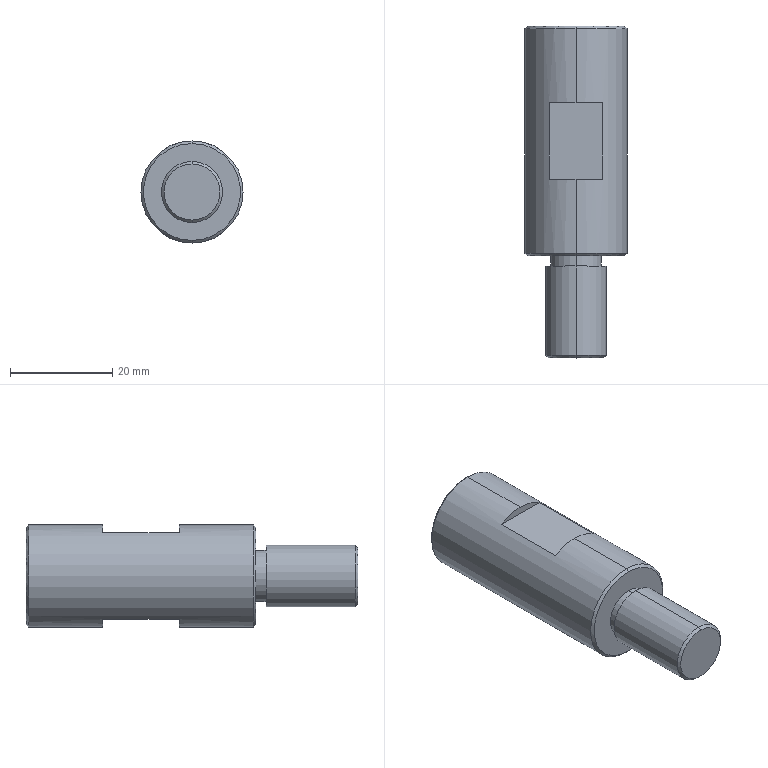Part | SolidWorks | features BaseBody 1 | 1 solid | 26 faces | box 20 x 65 x 20 mm | volume 14380 mm3 | plane 10 | cylinder 8 | cone 8 | commonest cylinder face diameters 8.5 x2 10 x2 12 x2 20 x2
STEP:
#1=CARTESIAN_POINT('',(0.,44.5,-10.));
#2=VERTEX_POINT('',#1);
#3=CARTESIAN_POINT('',(0.,44.5,10.));
#4=VERTEX_POINT('',#3);
#5=CARTESIAN_POINT('',(0.,44.5,0.));
#6=DIRECTION('',(0.,-1.,0.));
#7=DIRECTION('',(0.,0.,-1.));
#8=AXIS2_PLACEMENT_3D('',#5,#6,#7);
#9=CIRCLE('',#8,10.);
#10=EDGE_CURVE('',#2,#4,#9,.T.);
#11=ORIENTED_EDGE('',*,*,#10,.T.);
#12=CARTESIAN_POINT('',(0.,30.,10.));
#13=VERTEX_POINT('',#12);
#14=CARTESIAN_POINT('',(0.,45.,10.));
#15=DIRECTION('',(0.,-1.,0.));
#16=VECTOR('',#15,1000.);
#17=LINE('',#14,#16);
#18=EDGE_CURVE('',#4,#13,#17,.T.);
#19=ORIENTED_EDGE('',*,*,#18,.T.);
#20=CARTESIAN_POINT('',(5.268,30.,8.5));
#21=VERTEX_POINT('',#20);
#22=CARTESIAN_POINT('',(0.,30.,0.));
#23=DIRECTION('',(0.,1.,0.));
#24=DIRECTION('',(0.,0.,-1.));
#25=AXIS2_PLACEMENT_3D('',#22,#23,#24);
#26=CIRCLE('',#25,10.);
#27=EDGE_CURVE('',#13,#21,#26,.T.);
#28=ORIENTED_EDGE('',*,*,#27,.T.);
#29=CARTESIAN_POINT('',(5.268,15.,8.5));
#30=VERTEX_POINT('',#29);
#31=CARTESIAN_POINT('',(5.268,30.,8.5));
#32=DIRECTION('',(0.,-1.,0.));
#33=VECTOR('',#32,1000.);
#34=LINE('',#31,#33);
#35=EDGE_CURVE('',#21,#30,#34,.T.);
#36=ORIENTED_EDGE('',*,*,#35,.T.);
#37=CARTESIAN_POINT('',(0.,15.,10.));
#38=VERTEX_POINT('',#37);
#39=CARTESIAN_POINT('',(0.,15.,0.));
#40=DIRECTION('',(0.,-1.,0.));
#41=DIRECTION('',(0.,0.,-1.));
#42=AXIS2_PLACEMENT_3D('',#39,#40,#41);
#43=CIRCLE('',#42,10.);
#44=EDGE_CURVE('',#30,#38,#43,.T.);
#45=ORIENTED_EDGE('',*,*,#44,.T.);
#46=CARTESIAN_POINT('',(0.,0.5,10.));
#47=VERTEX_POINT('',#46);
#48=CARTESIAN_POINT('',(0.,45.,10.));
#49=DIRECTION('',(0.,-1.,0.));
#50=VECTOR('',#49,1000.);
#51=LINE('',#48,#50);
#52=EDGE_CURVE('',#38,#47,#51,.T.);
#53=ORIENTED_EDGE('',*,*,#52,.T.);
#54=CARTESIAN_POINT('',(0.,0.5,-10.));
#55=VERTEX_POINT('',#54);
#56=CARTESIAN_POINT('',(0.,0.5,0.));
#57=DIRECTION('',(0.,1.,0.));
#58=DIRECTION('',(0.,0.,-1.));
#59=AXIS2_PLACEMENT_3D('',#56,#57,#58);
#60=CIRCLE('',#59,10.);
#61=EDGE_CURVE('',#47,#55,#60,.T.);
#62=ORIENTED_EDGE('',*,*,#61,.T.);
#63=CARTESIAN_POINT('',(0.,15.,-10.));
#64=VERTEX_POINT('',#63);
#65=CARTESIAN_POINT('',(0.,45.,-10.));
#66=DIRECTION('',(0.,-1.,0.));
#67=VECTOR('',#66,1000.);
#68=LINE('',#65,#67);
#69=EDGE_CURVE('',#64,#55,#68,.T.);
#70=ORIENTED_EDGE('',*,*,#69,.F.);
#71=CARTESIAN_POINT('',(5.268,15.,-8.5));
#72=VERTEX_POINT('',#71);
#73=CARTESIAN_POINT('',(0.,15.,0.));
#74=DIRECTION('',(0.,-1.,0.));
#75=DIRECTION('',(0.,0.,-1.));
#76=AXIS2_PLACEMENT_3D('',#73,#74,#75);
#77=CIRCLE('',#76,10.);
#78=EDGE_CURVE('',#64,#72,#77,.T.);
#79=ORIENTED_EDGE('',*,*,#78,.T.);
#80=CARTESIAN_POINT('',(5.268,30.,-8.5));
#81=VERTEX_POINT('',#80);
#82=CARTESIAN_POINT('',(5.268,45.,-8.5));
#83=DIRECTION('',(0.,1.,0.));
#84=VECTOR('',#83,1000.);
#85=LINE('',#82,#84);
#86=EDGE_CURVE('',#72,#81,#85,.T.);
#87=ORIENTED_EDGE('',*,*,#86,.T.);
#88=CARTESIAN_POINT('',(0.,30.,-10.));
#89=VERTEX_POINT('',#88);
#90=CARTESIAN_POINT('',(0.,30.,0.));
#91=DIRECTION('',(0.,1.,0.));
#92=DIRECTION('',(0.,0.,-1.));
#93=AXIS2_PLACEMENT_3D('',#90,#91,#92);
#94=CIRCLE('',#93,10.);
#95=EDGE_CURVE('',#81,#89,#94,.T.);
#96=ORIENTED_EDGE('',*,*,#95,.T.);
#97=CARTESIAN_POINT('',(0.,45.,-10.));
#98=DIRECTION('',(0.,-1.,0.));
#99=VECTOR('',#98,1000.);
#100=LINE('',#97,#99);
#101=EDGE_CURVE('',#2,#89,#100,.T.);
#102=ORIENTED_EDGE('',*,*,#101,.F.);
#103=EDGE_LOOP('',(#11,#19,#28,#36,#45,#53,#62,#70,#79,#87,#96,#102));
#104=FACE_OUTER_BOUND('',#103,.T.);
#105=CARTESIAN_POINT('',(0.,45.,0.));
#106=DIRECTION('',(0.,-1.,0.));
#107=DIRECTION('',(0.,0.,-1.));
#108=AXIS2_PLACEMENT_3D('',#105,#106,#107);
#109=CYLINDRICAL_SURFACE('',#108,10.);
#110=ADVANCED_FACE('',(#104),#109,.T.);
#111=CARTESIAN_POINT('',(0.,0.,9.5));
#112=VERTEX_POINT('',#111);
#113=CARTESIAN_POINT('',(0.,0.,-9.5));
#114=VERTEX_POINT('',#113);
#115=CARTESIAN_POINT('',(0.,0.,0.));
#116=DIRECTION('',(0.,1.,0.));
#117=DIRECTION('',(0.,0.,1.));
#118=AXIS2_PLACEMENT_3D('',#115,#116,#117);
#119=CIRCLE('',#118,9.5);
#120=EDGE_CURVE('',#112,#114,#119,.T.);
#121=ORIENTED_EDGE('',*,*,#120,.T.);
#122=CARTESIAN_POINT('',(0.,0.5,-10.));
#123=DIRECTION('',(0.,0.7071,-0.7071));
#124=VECTOR('',#123,1000.);
#125=LINE('',#122,#124);
#126=EDGE_CURVE('',#114,#55,#125,.T.);
#127=ORIENTED_EDGE('',*,*,#126,.T.);
#128=ORIENTED_EDGE('',*,*,#61,.F.);
#129=CARTESIAN_POINT('',(0.,0.5,10.));
#130=DIRECTION('',(0.,0.7071,0.7071));
#131=VECTOR('',#130,1000.);
#132=LINE('',#129,#131);
#133=EDGE_CURVE('',#112,#47,#132,.T.);
#134=ORIENTED_EDGE('',*,*,#133,.F.);
#135=EDGE_LOOP('',(#121,#127,#128,#134));
#136=FACE_OUTER_BOUND('',#135,.T.);
#137=CARTESIAN_POINT('',(0.,0.5,0.));
#138=DIRECTION('',(0.,1.,0.));
#139=DIRECTION('',(0.,0.,1.));
#140=AXIS2_PLACEMENT_3D('',#137,#138,#139);
#141=CONICAL_SURFACE('',#140,10.,0.7854);
#142=ADVANCED_FACE('',(#136),#141,.T.);
#143=CARTESIAN_POINT('',(0.,45.,-9.5));
#144=VERTEX_POINT('',#143);
#145=CARTESIAN_POINT('',(0.,45.,9.5));
#146=VERTEX_POINT('',#145);
#147=CARTESIAN_POINT('',(0.,45.,0.));
#148=DIRECTION('',(0.,-1.,0.));
#149=DIRECTION('',(0.,0.,-1.));
#150=AXIS2_PLACEMENT_3D('',#147,#148,#149);
#151=CIRCLE('',#150,9.5);
#152=EDGE_CURVE('',#144,#146,#151,.T.);
#153=ORIENTED_EDGE('',*,*,#152,.T.);
#154=CARTESIAN_POINT('',(0.,44.5,10.));
#155=DIRECTION('',(0.,-0.7071,0.7071));
#156=VECTOR('',#155,1000.);
#157=LINE('',#154,#156);
#158=EDGE_CURVE('',#146,#4,#157,.T.);
#159=ORIENTED_EDGE('',*,*,#158,.T.);
#160=ORIENTED_EDGE('',*,*,#10,.F.);
#161=CARTESIAN_POINT('',(0.,44.5,-10.));
#162=DIRECTION('',(0.,-0.7071,-0.7071));
#163=VECTOR('',#162,1000.);
#164=LINE('',#161,#163);
#165=EDGE_CURVE('',#144,#2,#164,.T.);
#166=ORIENTED_EDGE('',*,*,#165,.F.);
#167=EDGE_LOOP('',(#153,#159,#160,#166));
#168=FACE_OUTER_BOUND('',#167,.T.);
#169=CARTESIAN_POINT('',(0.,44.5,0.));
#170=DIRECTION('',(0.,-1.,0.));
#171=DIRECTION('',(0.,0.,-1.));
#172=AXIS2_PLACEMENT_3D('',#169,#170,#171);
#173=CONICAL_SURFACE('',#172,10.,0.7854);
#174=ADVANCED_FACE('',(#168),#173,.T.);
#175=CARTESIAN_POINT('',(0.,-2.,5.));
#176=VERTEX_POINT('',#175);
#177=CARTESIAN_POINT('',(0.,-2.,-5.));
#178=VERTEX_POINT('',#177);
#179=CARTESIAN_POINT('',(0.,-2.,0.));
#180=DIRECTION('',(0.,1.,0.));
#181=DIRECTION('',(0.,0.,1.));
#182=AXIS2_PLACEMENT_3D('',#179,#180,#181);
#183=CIRCLE('',#182,5.);
#184=EDGE_CURVE('',#176,#178,#183,.T.);
#185=ORIENTED_EDGE('',*,*,#184,.T.);
#186=CARTESIAN_POINT('',(0.,0.,-5.));
#187=VERTEX_POINT('',#186);
#188=CARTESIAN_POINT('',(0.,-2.,-5.));
#189=DIRECTION('',(0.,1.,0.));
#190=VECTOR('',#189,1000.);
#191=LINE('',#188,#190);
#192=EDGE_CURVE('',#178,#187,#191,.T.);
#193=ORIENTED_EDGE('',*,*,#192,.T.);
#194=CARTESIAN_POINT('',(0.,0.,5.));
#195=VERTEX_POINT('',#194);
#196=CARTESIAN_POINT('',(0.,0.,0.));
#197=DIRECTION('',(0.,-1.,0.));
#198=DIRECTION('',(0.,0.,1.));
#199=AXIS2_PLACEMENT_3D('',#196,#197,#198);
#200=CIRCLE('',#199,5.);
#201=EDGE_CURVE('',#187,#195,#200,.T.);
#202=ORIENTED_EDGE('',*,*,#201,.T.);
#203=CARTESIAN_POINT('',(0.,-2.,5.));
#204=DIRECTION('',(0.,1.,0.));
#205=VECTOR('',#204,1000.);
#206=LINE('',#203,#205);
#207=EDGE_CURVE('',#176,#195,#206,.T.);
#208=ORIENTED_EDGE('',*,*,#207,.F.);
#209=EDGE_LOOP('',(#185,#193,#202,#208));
#210=FACE_OUTER_BOUND('',#209,.T.);
#211=CARTESIAN_POINT('',(0.,-2.,0.));
#212=DIRECTION('',(0.,1.,0.));
#213=DIRECTION('',(0.,0.,1.));
#214=AXIS2_PLACEMENT_3D('',#211,#212,#213);
#215=CYLINDRICAL_SURFACE('',#214,5.);
#216=ADVANCED_FACE('',(#210),#215,.T.);
#217=CARTESIAN_POINT('',(0.,17.5,-4.25));
#218=VERTEX_POINT('',#217);
#219=CARTESIAN_POINT('',(0.,17.5,4.25));
#220=VERTEX_POINT('',#219);
#221=CARTESIAN_POINT('',(0.,17.5,0.));
#222=DIRECTION('',(0.,1.,0.));
#223=DIRECTION('',(0.,0.,1.));
#224=AXIS2_PLACEMENT_3D('',#221,#222,#223);
#225=CIRCLE('',#224,4.25);
#226=EDGE_CURVE('',#218,#220,#225,.T.);
#227=ORIENTED_EDGE('',*,*,#226,.F.);
#228=CARTESIAN_POINT('',(0.,45.,-4.25));
#229=VERTEX_POINT('',#228);
#230=CARTESIAN_POINT('',(0.,45.,-4.25));
#231=DIRECTION('',(0.,1.,0.));
#232=VECTOR('',#231,1000.);
#233=LINE('',#230,#232);
#234=EDGE_CURVE('',#218,#229,#233,.T.);
#235=ORIENTED_EDGE('',*,*,#234,.T.);
#236=CARTESIAN_POINT('',(0.,45.,4.25));
#237=VERTEX_POINT('',#236);
#238=CARTESIAN_POINT('',(0.,45.,0.));
#239=DIRECTION('',(0.,-1.,0.));
#240=DIRECTION('',(0.,0.,1.));
#241=AXIS2_PLACEMENT_3D('',#238,#239,#240);
#242=CIRCLE('',#241,4.25);
#243=EDGE_CURVE('',#237,#229,#242,.T.);
#244=ORIENTED_EDGE('',*,*,#243,.F.);
#245=CARTESIAN_POINT('',(0.,45.,4.25));
#246=DIRECTION('',(0.,1.,0.));
#247=VECTOR('',#246,1000.);
#248=LINE('',#245,#247);
#249=EDGE_CURVE('',#220,#237,#248,.T.);
#250=ORIENTED_EDGE('',*,*,#249,.F.);
#251=EDGE_LOOP('',(#227,#235,#244,#250));
#252=FACE_OUTER_BOUND('',#251,.T.);
#253=CARTESIAN_POINT('',(0.,45.,0.));
#254=DIRECTION('',(0.,1.,0.));
#255=DIRECTION('',(0.,0.,1.));
#256=AXIS2_PLACEMENT_3D('',#253,#254,#255);
#257=CYLINDRICAL_SURFACE('',#256,4.25);
#258=ADVANCED_FACE('',(#252),#257,.F.);
#259=CARTESIAN_POINT('',(0.,14.946,0.));
#260=VERTEX_POINT('',#259);
#261=CARTESIAN_POINT('',(0.,17.5,4.25));
#262=DIRECTION('',(0.,0.515,0.8572));
#263=VECTOR('',#262,1000.);
#264=LINE('',#261,#263);
#265=EDGE_CURVE('',#260,#220,#264,.T.);
#266=ORIENTED_EDGE('',*,*,#265,.F.);
#267=CARTESIAN_POINT('',(0.,17.5,-4.25));
#268=DIRECTION('',(0.,0.515,-0.8572));
#269=VECTOR('',#268,1000.);
#270=LINE('',#267,#269);
#271=EDGE_CURVE('',#260,#218,#270,.T.);
#272=ORIENTED_EDGE('',*,*,#271,.T.);
#273=ORIENTED_EDGE('',*,*,#226,.T.);
#274=EDGE_LOOP('',(#266,#272,#273));
#275=FACE_OUTER_BOUND('',#274,.T.);
#276=CARTESIAN_POINT('',(0.,17.5,0.));
#277=DIRECTION('',(0.,1.,0.));
#278=DIRECTION('',(0.,0.,1.));
#279=AXIS2_PLACEMENT_3D('',#276,#277,#278);
#280=CONICAL_SURFACE('',#279,4.25,1.03);
#281=ADVANCED_FACE('',(#275),#280,.F.);
#282=CARTESIAN_POINT('',(0.,-19.5,6.));
#283=VERTEX_POINT('',#282);
#284=CARTESIAN_POINT('',(0.,-19.5,-6.));
#285=VERTEX_POINT('',#284);
#286=CARTESIAN_POINT('',(0.,-19.5,0.));
#287=DIRECTION('',(0.,1.,0.));
#288=DIRECTION('',(0.,0.,1.));
#289=AXIS2_PLACEMENT_3D('',#286,#287,#288);
#290=CIRCLE('',#289,6.);
#291=EDGE_CURVE('',#283,#285,#290,.T.);
#292=ORIENTED_EDGE('',*,*,#291,.T.);
#293=CARTESIAN_POINT('',(0.,-2.,-6.));
#294=VERTEX_POINT('',#293);
#295=CARTESIAN_POINT('',(0.,-20.,-6.));
#296=DIRECTION('',(0.,1.,0.));
#297=VECTOR('',#296,1000.);
#298=LINE('',#295,#297);
#299=EDGE_CURVE('',#285,#294,#298,.T.);
#300=ORIENTED_EDGE('',*,*,#299,.T.);
#301=CARTESIAN_POINT('',(0.,-2.,6.));
#302=VERTEX_POINT('',#301);
#303=CARTESIAN_POINT('',(0.,-2.,0.));
#304=DIRECTION('',(0.,-1.,0.));
#305=DIRECTION('',(0.,0.,1.));
#306=AXIS2_PLACEMENT_3D('',#303,#304,#305);
#307=CIRCLE('',#306,6.);
#308=EDGE_CURVE('',#294,#302,#307,.T.);
#309=ORIENTED_EDGE('',*,*,#308,.T.);
#310=CARTESIAN_POINT('',(0.,-20.,6.));
#311=DIRECTION('',(0.,1.,0.));
#312=VECTOR('',#311,1000.);
#313=LINE('',#310,#312);
#314=EDGE_CURVE('',#283,#302,#313,.T.);
#315=ORIENTED_EDGE('',*,*,#314,.F.);
#316=EDGE_LOOP('',(#292,#300,#309,#315));
#317=FACE_OUTER_BOUND('',#316,.T.);
#318=CARTESIAN_POINT('',(0.,-20.,0.));
#319=DIRECTION('',(0.,1.,0.));
#320=DIRECTION('',(0.,0.,1.));
#321=AXIS2_PLACEMENT_3D('',#318,#319,#320);
#322=CYLINDRICAL_SURFACE('',#321,6.);
#323=ADVANCED_FACE('',(#317),#322,.T.);
#324=CARTESIAN_POINT('',(0.,-20.,5.5));
#325=VERTEX_POINT('',#324);
#326=CARTESIAN_POINT('',(0.,-20.,-5.5));
#327=VERTEX_POINT('',#326);
#328=CARTESIAN_POINT('',(0.,-20.,0.));
#329=DIRECTION('',(0.,1.,0.));
#330=DIRECTION('',(0.,0.,1.));
#331=AXIS2_PLACEMENT_3D('',#328,#329,#330);
#332=CIRCLE('',#331,5.5);
#333=EDGE_CURVE('',#325,#327,#332,.T.);
#334=ORIENTED_EDGE('',*,*,#333,.T.);
#335=CARTESIAN_POINT('',(0.,-19.5,-6.));
#336=DIRECTION('',(0.,0.7071,-0.7071));
#337=VECTOR('',#336,1000.);
#338=LINE('',#335,#337);
#339=EDGE_CURVE('',#327,#285,#338,.T.);
#340=ORIENTED_EDGE('',*,*,#339,.T.);
#341=ORIENTED_EDGE('',*,*,#291,.F.);
#342=CARTESIAN_POINT('',(0.,-19.5,6.));
#343=DIRECTION('',(0.,0.7071,0.7071));
#344=VECTOR('',#343,1000.);
#345=LINE('',#342,#344);
#346=EDGE_CURVE('',#325,#283,#345,.T.);
#347=ORIENTED_EDGE('',*,*,#346,.F.);
#348=EDGE_LOOP('',(#334,#340,#341,#347));
#349=FACE_OUTER_BOUND('',#348,.T.);
#350=CARTESIAN_POINT('',(0.,-19.5,0.));
#351=DIRECTION('',(0.,1.,0.));
#352=DIRECTION('',(0.,0.,1.));
#353=AXIS2_PLACEMENT_3D('',#350,#351,#352);
#354=CONICAL_SURFACE('',#353,6.,0.7854);
#355=ADVANCED_FACE('',(#349),#354,.T.);
#356=ORIENTED_EDGE('',*,*,#18,.F.);
#357=CARTESIAN_POINT('',(0.,44.5,0.));
#358=DIRECTION('',(0.,-1.,0.));
#359=DIRECTION('',(0.,0.,-1.));
#360=AXIS2_PLACEMENT_3D('',#357,#358,#359);
#361=CIRCLE('',#360,10.);
#362=EDGE_CURVE('',#4,#2,#361,.T.);
#363=ORIENTED_EDGE('',*,*,#362,.T.);
#364=ORIENTED_EDGE('',*,*,#101,.T.);
#365=CARTESIAN_POINT('',(-5.268,30.,-8.5));
#366=VERTEX_POINT('',#365);
#367=CARTESIAN_POINT('',(0.,30.,0.));
#368=DIRECTION('',(0.,1.,0.));
#369=DIRECTION('',(0.,0.,-1.));
#370=AXIS2_PLACEMENT_3D('',#367,#368,#369);
#371=CIRCLE('',#370,10.);
#372=EDGE_CURVE('',#89,#366,#371,.T.);
#373=ORIENTED_EDGE('',*,*,#372,.T.);
#374=CARTESIAN_POINT('',(-5.268,15.,-8.5));
#375=VERTEX_POINT('',#374);
#376=CARTESIAN_POINT('',(-5.268,45.,-8.5));
#377=DIRECTION('',(0.,-1.,0.));
#378=VECTOR('',#377,1000.);
#379=LINE('',#376,#378);
#380=EDGE_CURVE('',#366,#375,#379,.T.);
#381=ORIENTED_EDGE('',*,*,#380,.T.);
#382=CARTESIAN_POINT('',(0.,15.,0.));
#383=DIRECTION('',(0.,-1.,0.));
#384=DIRECTION('',(0.,0.,-1.));
#385=AXIS2_PLACEMENT_3D('',#382,#383,#384);
#386=CIRCLE('',#385,10.);
#387=EDGE_CURVE('',#375,#64,#386,.T.);
#388=ORIENTED_EDGE('',*,*,#387,.T.);
#389=ORIENTED_EDGE('',*,*,#69,.T.);
#390=CARTESIAN_POINT('',(0.,0.5,0.));
#391=DIRECTION('',(0.,1.,0.));
#392=DIRECTION('',(0.,0.,-1.));
#393=AXIS2_PLACEMENT_3D('',#390,#391,#392);
#394=CIRCLE('',#393,10.);
#395=EDGE_CURVE('',#55,#47,#394,.T.);
#396=ORIENTED_EDGE('',*,*,#395,.T.);
#397=ORIENTED_EDGE('',*,*,#52,.F.);
#398=CARTESIAN_POINT('',(-5.268,15.,8.5));
#399=VERTEX_POINT('',#398);
#400=CARTESIAN_POINT('',(0.,15.,0.));
#401=DIRECTION('',(0.,-1.,0.));
#402=DIRECTION('',(0.,0.,-1.));
#403=AXIS2_PLACEMENT_3D('',#400,#401,#402);
#404=CIRCLE('',#403,10.);
#405=EDGE_CURVE('',#38,#399,#404,.T.);
#406=ORIENTED_EDGE('',*,*,#405,.T.);
#407=CARTESIAN_POINT('',(-5.268,30.,8.5));
#408=VERTEX_POINT('',#407);
#409=CARTESIAN_POINT('',(-5.268,45.,8.5));
#410=DIRECTION('',(0.,1.,0.));
#411=VECTOR('',#410,1000.);
#412=LINE('',#409,#411);
#413=EDGE_CURVE('',#399,#408,#412,.T.);
#414=ORIENTED_EDGE('',*,*,#413,.T.);
#415=CARTESIAN_POINT('',(0.,30.,0.));
#416=DIRECTION('',(0.,1.,0.));
#417=DIRECTION('',(0.,0.,-1.));
#418=AXIS2_PLACEMENT_3D('',#415,#416,#417);
#419=CIRCLE('',#418,10.);
#420=EDGE_CURVE('',#408,#13,#419,.T.);
#421=ORIENTED_EDGE('',*,*,#420,.T.);
#422=EDGE_LOOP('',(#356,#363,#364,#373,#381,#388,#389,#396,#397,#406,#414,#421));
#423=FACE_OUTER_BOUND('',#422,.T.);
#424=CARTESIAN_POINT('',(0.,45.,0.));
#425=DIRECTION('',(0.,-1.,0.));
#426=DIRECTION('',(0.,0.,-1.));
#427=AXIS2_PLACEMENT_3D('',#424,#425,#426);
#428=CYLINDRICAL_SURFACE('',#427,10.);
#429=ADVANCED_FACE('',(#423),#428,.T.);
#430=CARTESIAN_POINT('',(0.,30.,8.5));
#431=DIRECTION('',(-1.,0.,0.));
#432=VECTOR('',#431,1000.);
#433=LINE('',#430,#432);
#434=EDGE_CURVE('',#21,#408,#433,.T.);
#435=ORIENTED_EDGE('',*,*,#434,.F.);
#436=ORIENTED_EDGE('',*,*,#27,.F.);
#437=ORIENTED_EDGE('',*,*,#420,.F.);
#438=EDGE_LOOP('',(#435,#436,#437));
#439=FACE_OUTER_BOUND('',#438,.T.);
#440=CARTESIAN_POINT('',(0.,30.,0.));
#441=DIRECTION('',(0.,1.,0.));
#442=DIRECTION('',(0.,0.,1.));
#443=AXIS2_PLACEMENT_3D('',#440,#441,#442);
#444=PLANE('',#443);
#445=ADVANCED_FACE('',(#439),#444,.F.);
#446=ORIENTED_EDGE('',*,*,#413,.F.);
#447=CARTESIAN_POINT('',(-16.025,15.,8.5));
#448=DIRECTION('',(-1.,0.,0.));
#449=VECTOR('',#448,1000.);
#450=LINE('',#447,#449);
#451=EDGE_CURVE('',#30,#399,#450,.T.);
#452=ORIENTED_EDGE('',*,*,#451,.F.);
#453=ORIENTED_EDGE('',*,*,#35,.F.);
#454=ORIENTED_EDGE('',*,*,#434,.T.);
#455=EDGE_LOOP('',(#446,#452,#453,#454));
#456=FACE_OUTER_BOUND('',#455,.T.);
#457=CARTESIAN_POINT('',(-16.025,30.,8.5));
#458=DIRECTION('',(0.,0.,-1.));
#459=DIRECTION('',(-1.,0.,0.));
#460=AXIS2_PLACEMENT_3D('',#457,#458,#459);
#461=PLANE('',#460);
#462=ADVANCED_FACE('',(#456),#461,.F.);
#463=ORIENTED_EDGE('',*,*,#44,.F.);
#464=ORIENTED_EDGE('',*,*,#451,.T.);
#465=ORIENTED_EDGE('',*,*,#405,.F.);
#466=EDGE_LOOP('',(#463,#464,#465));
#467=FACE_OUTER_BOUND('',#466,.T.);
#468=CARTESIAN_POINT('',(0.,15.,0.));
#469=DIRECTION('',(0.,1.,0.));
#470=DIRECTION('',(0.,0.,1.));
#471=AXIS2_PLACEMENT_3D('',#468,#469,#470);
#472=PLANE('',#471);
#473=ADVANCED_FACE('',(#467),#472,.T.);
#474=ORIENTED_EDGE('',*,*,#126,.F.);
#475=CARTESIAN_POINT('',(0.,0.,0.));
#476=DIRECTION('',(0.,1.,0.));
#477=DIRECTION('',(0.,0.,1.));
#478=AXIS2_PLACEMENT_3D('',#475,#476,#477);
#479=CIRCLE('',#478,9.5);
#480=EDGE_CURVE('',#114,#112,#479,.T.);
#481=ORIENTED_EDGE('',*,*,#480,.T.);
#482=ORIENTED_EDGE('',*,*,#133,.T.);
#483=ORIENTED_EDGE('',*,*,#395,.F.);
#484=EDGE_LOOP('',(#474,#481,#482,#483));
#485=FACE_OUTER_BOUND('',#484,.T.);
#486=CARTESIAN_POINT('',(0.,0.5,0.));
#487=DIRECTION('',(0.,1.,0.));
#488=DIRECTION('',(0.,0.,1.));
#489=AXIS2_PLACEMENT_3D('',#486,#487,#488);
#490=CONICAL_SURFACE('',#489,10.,0.7854);
#491=ADVANCED_FACE('',(#485),#490,.T.);
#492=ORIENTED_EDGE('',*,*,#387,.F.);
#493=CARTESIAN_POINT('',(0.,15.,-8.5));
#494=DIRECTION('',(1.,0.,0.));
#495=VECTOR('',#494,1000.);
#496=LINE('',#493,#495);
#497=EDGE_CURVE('',#375,#72,#496,.T.);
#498=ORIENTED_EDGE('',*,*,#497,.T.);
#499=ORIENTED_EDGE('',*,*,#78,.F.);
#500=EDGE_LOOP('',(#492,#498,#499));
#501=FACE_OUTER_BOUND('',#500,.T.);
#502=CARTESIAN_POINT('',(0.,15.,0.));
#503=DIRECTION('',(0.,1.,0.));
#504=DIRECTION('',(0.,0.,1.));
#505=AXIS2_PLACEMENT_3D('',#502,#503,#504);
#506=PLANE('',#505);
#507=ADVANCED_FACE('',(#501),#506,.T.);
#508=ORIENTED_EDGE('',*,*,#86,.F.);
#509=ORIENTED_EDGE('',*,*,#497,.F.);
#510=ORIENTED_EDGE('',*,*,#380,.F.);
#511=CARTESIAN_POINT('',(-16.025,30.,-8.5));
#512=DIRECTION('',(-1.,0.,0.));
#513=VECTOR('',#512,1000.);
#514=LINE('',#511,#513);
#515=EDGE_CURVE('',#81,#366,#514,.T.);
#516=ORIENTED_EDGE('',*,*,#515,.F.);
#517=EDGE_LOOP('',(#508,#509,#510,#516));
#518=FACE_OUTER_BOUND('',#517,.T.);
#519=CARTESIAN_POINT('',(-16.025,30.,-8.5));
#520=DIRECTION('',(0.,0.,1.));
#521=DIRECTION('',(1.,0.,0.));
#522=AXIS2_PLACEMENT_3D('',#519,#520,#521);
#523=PLANE('',#522);
#524=ADVANCED_FACE('',(#518),#523,.F.);
#525=ORIENTED_EDGE('',*,*,#95,.F.);
#526=ORIENTED_EDGE('',*,*,#515,.T.);
#527=ORIENTED_EDGE('',*,*,#372,.F.);
#528=EDGE_LOOP('',(#525,#526,#527));
#529=FACE_OUTER_BOUND('',#528,.T.);
#530=CARTESIAN_POINT('',(0.,30.,0.));
#531=DIRECTION('',(0.,1.,0.));
#532=DIRECTION('',(0.,0.,1.));
#533=AXIS2_PLACEMENT_3D('',#530,#531,#532);
#534=PLANE('',#533);
#535=ADVANCED_FACE('',(#529),#534,.F.);
#536=ORIENTED_EDGE('',*,*,#158,.F.);
#537=CARTESIAN_POINT('',(0.,45.,0.));
#538=DIRECTION('',(0.,-1.,0.));
#539=DIRECTION('',(0.,0.,-1.));
#540=AXIS2_PLACEMENT_3D('',#537,#538,#539);
#541=CIRCLE('',#540,9.5);
#542=EDGE_CURVE('',#146,#144,#541,.T.);
#543=ORIENTED_EDGE('',*,*,#542,.T.);
#544=ORIENTED_EDGE('',*,*,#165,.T.);
#545=ORIENTED_EDGE('',*,*,#362,.F.);
#546=EDGE_LOOP('',(#536,#543,#544,#545));
#547=FACE_OUTER_BOUND('',#546,.T.);
#548=CARTESIAN_POINT('',(0.,44.5,0.));
#549=DIRECTION('',(0.,-1.,0.));
#550=DIRECTION('',(0.,0.,-1.));
#551=AXIS2_PLACEMENT_3D('',#548,#549,#550);
#552=CONICAL_SURFACE('',#551,10.,0.7854);
#553=ADVANCED_FACE('',(#547),#552,.T.);
#554=CARTESIAN_POINT('',(0.,0.,0.));
#555=DIRECTION('',(0.,-1.,0.));
#556=DIRECTION('',(0.,0.,1.));
#557=AXIS2_PLACEMENT_3D('',#554,#555,#556);
#558=CIRCLE('',#557,5.);
#559=EDGE_CURVE('',#195,#187,#558,.T.);
#560=ORIENTED_EDGE('',*,*,#559,.F.);
#561=ORIENTED_EDGE('',*,*,#201,.F.);
#562=EDGE_LOOP('',(#560,#561));
#563=FACE_BOUND('',#562,.T.);
#564=ORIENTED_EDGE('',*,*,#120,.F.);
#565=ORIENTED_EDGE('',*,*,#480,.F.);
#566=EDGE_LOOP('',(#564,#565));
#567=FACE_OUTER_BOUND('',#566,.T.);
#568=CARTESIAN_POINT('',(0.,0.,0.));
#569=DIRECTION('',(0.,1.,0.));
#570=DIRECTION('',(0.,0.,1.));
#571=AXIS2_PLACEMENT_3D('',#568,#569,#570);
#572=PLANE('',#571);
#573=ADVANCED_FACE('',(#563,#567),#572,.F.);
#574=ORIENTED_EDGE('',*,*,#243,.T.);
#575=CARTESIAN_POINT('',(0.,45.,0.));
#576=DIRECTION('',(0.,-1.,0.));
#577=DIRECTION('',(0.,0.,1.));
#578=AXIS2_PLACEMENT_3D('',#575,#576,#577);
#579=CIRCLE('',#578,4.25);
#580=EDGE_CURVE('',#229,#237,#579,.T.);
#581=ORIENTED_EDGE('',*,*,#580,.T.);
#582=EDGE_LOOP('',(#574,#581));
#583=FACE_BOUND('',#582,.T.);
#584=ORIENTED_EDGE('',*,*,#152,.F.);
#585=ORIENTED_EDGE('',*,*,#542,.F.);
#586=EDGE_LOOP('',(#584,#585));
#587=FACE_OUTER_BOUND('',#586,.T.);
#588=CARTESIAN_POINT('',(0.,45.,0.));
#589=DIRECTION('',(0.,1.,0.));
#590=DIRECTION('',(0.,0.,1.));
#591=AXIS2_PLACEMENT_3D('',#588,#589,#590);
#592=PLANE('',#591);
#593=ADVANCED_FACE('',(#583,#587),#592,.T.);
#594=ORIENTED_EDGE('',*,*,#192,.F.);
#595=CARTESIAN_POINT('',(0.,-2.,0.));
#596=DIRECTION('',(0.,1.,0.));
#597=DIRECTION('',(0.,0.,1.));
#598=AXIS2_PLACEMENT_3D('',#595,#596,#597);
#599=CIRCLE('',#598,5.);
#600=EDGE_CURVE('',#178,#176,#599,.T.);
#601=ORIENTED_EDGE('',*,*,#600,.T.);
#602=ORIENTED_EDGE('',*,*,#207,.T.);
#603=ORIENTED_EDGE('',*,*,#559,.T.);
#604=EDGE_LOOP('',(#594,#601,#602,#603));
#605=FACE_OUTER_BOUND('',#604,.T.);
#606=CARTESIAN_POINT('',(0.,-2.,0.));
#607=DIRECTION('',(0.,1.,0.));
#608=DIRECTION('',(0.,0.,1.));
#609=AXIS2_PLACEMENT_3D('',#606,#607,#608);
#610=CYLINDRICAL_SURFACE('',#609,5.);
#611=ADVANCED_FACE('',(#605),#610,.T.);
#612=ORIENTED_EDGE('',*,*,#234,.F.);
#613=CARTESIAN_POINT('',(0.,17.5,0.));
#614=DIRECTION('',(0.,1.,0.));
#615=DIRECTION('',(0.,0.,1.));
#616=AXIS2_PLACEMENT_3D('',#613,#614,#615);
#617=CIRCLE('',#616,4.25);
#618=EDGE_CURVE('',#220,#218,#617,.T.);
#619=ORIENTED_EDGE('',*,*,#618,.F.);
#620=ORIENTED_EDGE('',*,*,#249,.T.);
#621=ORIENTED_EDGE('',*,*,#580,.F.);
#622=EDGE_LOOP('',(#612,#619,#620,#621));
#623=FACE_OUTER_BOUND('',#622,.T.);
#624=CARTESIAN_POINT('',(0.,45.,0.));
#625=DIRECTION('',(0.,1.,0.));
#626=DIRECTION('',(0.,0.,1.));
#627=AXIS2_PLACEMENT_3D('',#624,#625,#626);
#628=CYLINDRICAL_SURFACE('',#627,4.25);
#629=ADVANCED_FACE('',(#623),#628,.F.);
#630=CARTESIAN_POINT('',(0.,-2.,0.));
#631=DIRECTION('',(0.,-1.,0.));
#632=DIRECTION('',(0.,0.,1.));
#633=AXIS2_PLACEMENT_3D('',#630,#631,#632);
#634=CIRCLE('',#633,6.);
#635=EDGE_CURVE('',#302,#294,#634,.T.);
#636=ORIENTED_EDGE('',*,*,#635,.F.);
#637=ORIENTED_EDGE('',*,*,#308,.F.);
#638=EDGE_LOOP('',(#636,#637));
#639=FACE_OUTER_BOUND('',#638,.T.);
#640=ORIENTED_EDGE('',*,*,#184,.F.);
#641=ORIENTED_EDGE('',*,*,#600,.F.);
#642=EDGE_LOOP('',(#640,#641));
#643=FACE_BOUND('',#642,.T.);
#644=CARTESIAN_POINT('',(0.,-2.,0.));
#645=DIRECTION('',(0.,-1.,0.));
#646=DIRECTION('',(0.,0.,-1.));
#647=AXIS2_PLACEMENT_3D('',#644,#645,#646);
#648=PLANE('',#647);
#649=ADVANCED_FACE('',(#639,#643),#648,.F.);
#650=ORIENTED_EDGE('',*,*,#271,.F.);
#651=ORIENTED_EDGE('',*,*,#265,.T.);
#652=ORIENTED_EDGE('',*,*,#618,.T.);
#653=EDGE_LOOP('',(#650,#651,#652));
#654=FACE_OUTER_BOUND('',#653,.T.);
#655=CARTESIAN_POINT('',(0.,17.5,0.));
#656=DIRECTION('',(0.,1.,0.));
#657=DIRECTION('',(0.,0.,1.));
#658=AXIS2_PLACEMENT_3D('',#655,#656,#657);
#659=CONICAL_SURFACE('',#658,4.25,1.03);
#660=ADVANCED_FACE('',(#654),#659,.F.);
#661=ORIENTED_EDGE('',*,*,#299,.F.);
#662=CARTESIAN_POINT('',(0.,-19.5,0.));
#663=DIRECTION('',(0.,1.,0.));
#664=DIRECTION('',(0.,0.,1.));
#665=AXIS2_PLACEMENT_3D('',#662,#663,#664);
#666=CIRCLE('',#665,6.);
#667=EDGE_CURVE('',#285,#283,#666,.T.);
#668=ORIENTED_EDGE('',*,*,#667,.T.);
#669=ORIENTED_EDGE('',*,*,#314,.T.);
#670=ORIENTED_EDGE('',*,*,#635,.T.);
#671=EDGE_LOOP('',(#661,#668,#669,#670));
#672=FACE_OUTER_BOUND('',#671,.T.);
#673=CARTESIAN_POINT('',(0.,-20.,0.));
#674=DIRECTION('',(0.,1.,0.));
#675=DIRECTION('',(0.,0.,1.));
#676=AXIS2_PLACEMENT_3D('',#673,#674,#675);
#677=CYLINDRICAL_SURFACE('',#676,6.);
#678=ADVANCED_FACE('',(#672),#677,.T.);
#679=ORIENTED_EDGE('',*,*,#339,.F.);
#680=CARTESIAN_POINT('',(0.,-20.,0.));
#681=DIRECTION('',(0.,1.,0.));
#682=DIRECTION('',(0.,0.,1.));
#683=AXIS2_PLACEMENT_3D('',#680,#681,#682);
#684=CIRCLE('',#683,5.5);
#685=EDGE_CURVE('',#327,#325,#684,.T.);
#686=ORIENTED_EDGE('',*,*,#685,.T.);
#687=ORIENTED_EDGE('',*,*,#346,.T.);
#688=ORIENTED_EDGE('',*,*,#667,.F.);
#689=EDGE_LOOP('',(#679,#686,#687,#688));
#690=FACE_OUTER_BOUND('',#689,.T.);
#691=CARTESIAN_POINT('',(0.,-19.5,0.));
#692=DIRECTION('',(0.,1.,0.));
#693=DIRECTION('',(0.,0.,1.));
#694=AXIS2_PLACEMENT_3D('',#691,#692,#693);
#695=CONICAL_SURFACE('',#694,6.,0.7854);
#696=ADVANCED_FACE('',(#690),#695,.T.);
#697=ORIENTED_EDGE('',*,*,#333,.F.);
#698=ORIENTED_EDGE('',*,*,#685,.F.);
#699=EDGE_LOOP('',(#697,#698));
#700=FACE_OUTER_BOUND('',#699,.T.);
#701=CARTESIAN_POINT('',(0.,-20.,0.));
#702=DIRECTION('',(0.,-1.,0.));
#703=DIRECTION('',(0.,0.,-1.));
#704=AXIS2_PLACEMENT_3D('',#701,#702,#703);
#705=PLANE('',#704);
#706=ADVANCED_FACE('',(#700),#705,.T.);
#707=CLOSED_SHELL('',(#110,#142,#174,#216,#258,#281,#323,#355,#429,#445,#462,#473,#491,#507,#524,#535,#553,#573,#593,#611,#629,#649,#660,#678,#696,#706));
#708=MANIFOLD_SOLID_BREP('',#707);
#709=CARTESIAN_POINT('',(0.,0.,0.));
#710=DIRECTION('',(0.,0.,1.));
#711=DIRECTION('',(1.,0.,0.));
#712=AXIS2_PLACEMENT_3D('',#709,#710,#711);
#713=(LENGTH_UNIT()NAMED_UNIT(*)SI_UNIT(.MILLI.,.METRE.));
#714=UNCERTAINTY_MEASURE_WITH_UNIT(LENGTH_MEASURE(0.00001),#713,'','');
#715=(NAMED_UNIT(*)PLANE_ANGLE_UNIT()SI_UNIT($,.RADIAN.));
#716=(NAMED_UNIT(*)SI_UNIT($,.STERADIAN.)SOLID_ANGLE_UNIT());
#717=(GEOMETRIC_REPRESENTATION_CONTEXT(3)GLOBAL_UNCERTAINTY_ASSIGNED_CONTEXT((#714))GLOBAL_UNIT_ASSIGNED_CONTEXT((#713,#715,#716))REPRESENTATION_CONTEXT('',''));
#718=ADVANCED_BREP_SHAPE_REPRESENTATION('',(#708,#712),#717);